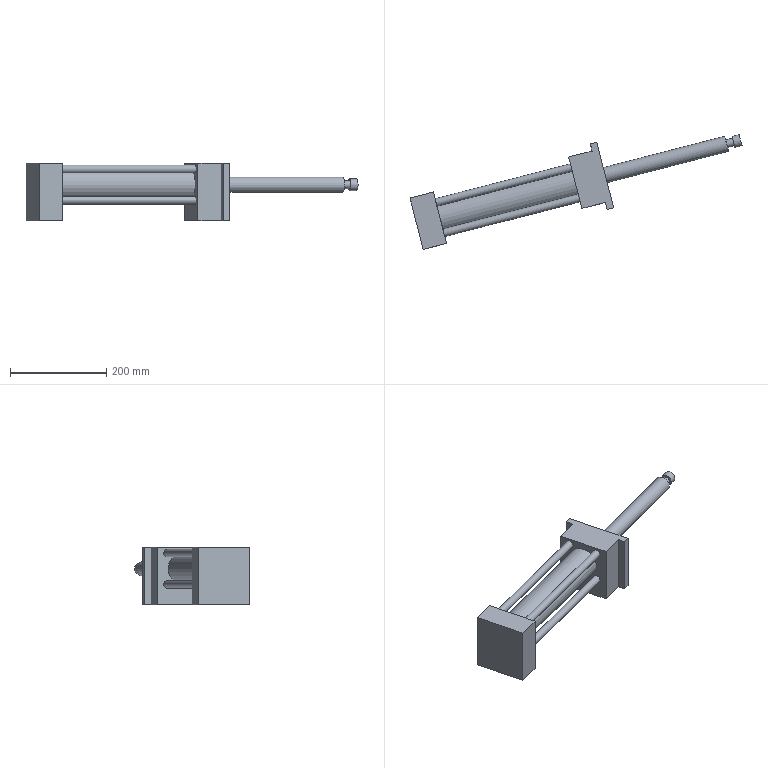Part | STEP file | 车灯-后视镜_id422_x_t | 1 solid | 27 faces | box 688.746 x 238.169 x 120 mm | volume 2911913 mm3 | plane 19 | cylinder 8 | commonest cylinder face diameters 16 x5 24 x1 32 x1 63 x1
STEP:
#1=CARTESIAN_POINT('',(-879.412,-211.845,49.5));
#2=VERTEX_POINT('',#1);
#3=CARTESIAN_POINT('',(-879.412,-211.845,-70.5));
#4=VERTEX_POINT('',#3);
#5=CARTESIAN_POINT('',(-879.412,-211.845,-110.845));
#6=DIRECTION('',(0.,0.,-1.));
#7=VECTOR('',#6,1.);
#8=LINE('',#5,#7);
#9=EDGE_CURVE('',#2,#4,#8,.T.);
#10=ORIENTED_EDGE('',*,*,#9,.T.);
#11=CARTESIAN_POINT('',(-830.995,-199.36,-70.5));
#12=VERTEX_POINT('',#11);
#13=CARTESIAN_POINT('',(-400.091,-88.244,-70.5));
#14=DIRECTION('',(0.9683,0.2497,0.));
#15=VECTOR('',#14,1.);
#16=LINE('',#13,#15);
#17=EDGE_CURVE('',#4,#12,#16,.T.);
#18=ORIENTED_EDGE('',*,*,#17,.T.);
#19=CARTESIAN_POINT('',(-830.995,-199.36,49.5));
#20=VERTEX_POINT('',#19);
#21=CARTESIAN_POINT('',(-830.995,-199.36,-110.845));
#22=DIRECTION('',(0.,0.,-1.));
#23=VECTOR('',#22,1.);
#24=LINE('',#21,#23);
#25=EDGE_CURVE('',#20,#12,#24,.T.);
#26=ORIENTED_EDGE('',*,*,#25,.F.);
#27=CARTESIAN_POINT('',(-400.091,-88.244,49.5));
#28=DIRECTION('',(0.9683,0.2497,0.));
#29=VECTOR('',#28,1.);
#30=LINE('',#27,#29);
#31=EDGE_CURVE('',#2,#20,#30,.T.);
#32=ORIENTED_EDGE('',*,*,#31,.F.);
#33=EDGE_LOOP('',(#10,#18,#26,#32));
#34=FACE_OUTER_BOUND('',#33,.T.);
#35=CARTESIAN_POINT('',(-545.34,-125.699,-110.845));
#36=DIRECTION('',(-0.2497,0.9683,0.));
#37=DIRECTION('',(0.,0.,-1.));
#38=AXIS2_PLACEMENT_3D('',#35,#36,#37);
#39=PLANE('',#38);
#40=ADVANCED_FACE('',(#34),#39,.F.);
#41=CARTESIAN_POINT('',(-906.878,-105.329,49.5));
#42=VERTEX_POINT('',#41);
#43=CARTESIAN_POINT('',(-858.462,-92.844,49.5));
#44=VERTEX_POINT('',#43);
#45=CARTESIAN_POINT('',(-427.558,18.272,49.5));
#46=DIRECTION('',(0.9683,0.2497,0.));
#47=VECTOR('',#46,1.);
#48=LINE('',#45,#47);
#49=EDGE_CURVE('',#42,#44,#48,.T.);
#50=ORIENTED_EDGE('',*,*,#49,.T.);
#51=CARTESIAN_POINT('',(-858.462,-92.844,-70.5));
#52=VERTEX_POINT('',#51);
#53=CARTESIAN_POINT('',(-858.462,-92.844,-110.845));
#54=DIRECTION('',(0.,0.,-1.));
#55=VECTOR('',#54,1.);
#56=LINE('',#53,#55);
#57=EDGE_CURVE('',#44,#52,#56,.T.);
#58=ORIENTED_EDGE('',*,*,#57,.T.);
#59=CARTESIAN_POINT('',(-906.878,-105.329,-70.5));
#60=VERTEX_POINT('',#59);
#61=CARTESIAN_POINT('',(-427.558,18.272,-70.5));
#62=DIRECTION('',(0.9683,0.2497,0.));
#63=VECTOR('',#62,1.);
#64=LINE('',#61,#63);
#65=EDGE_CURVE('',#60,#52,#64,.T.);
#66=ORIENTED_EDGE('',*,*,#65,.F.);
#67=CARTESIAN_POINT('',(-906.878,-105.329,-110.845));
#68=DIRECTION('',(0.,0.,-1.));
#69=VECTOR('',#68,1.);
#70=LINE('',#67,#69);
#71=EDGE_CURVE('',#42,#60,#70,.T.);
#72=ORIENTED_EDGE('',*,*,#71,.F.);
#73=EDGE_LOOP('',(#50,#58,#66,#72));
#74=FACE_OUTER_BOUND('',#73,.T.);
#75=CARTESIAN_POINT('',(-572.807,-19.183,-110.845));
#76=DIRECTION('',(-0.2497,0.9683,0.));
#77=DIRECTION('',(0.,0.,-1.));
#78=AXIS2_PLACEMENT_3D('',#75,#76,#77);
#79=PLANE('',#78);
#80=ADVANCED_FACE('',(#74),#79,.T.);
#81=ORIENTED_EDGE('',*,*,#31,.T.);
#82=CARTESIAN_POINT('',(-844.729,-146.102,49.5));
#83=DIRECTION('',(-0.2497,0.9683,0.));
#84=VECTOR('',#83,1.);
#85=LINE('',#82,#84);
#86=EDGE_CURVE('',#20,#44,#85,.T.);
#87=ORIENTED_EDGE('',*,*,#86,.T.);
#88=ORIENTED_EDGE('',*,*,#49,.F.);
#89=CARTESIAN_POINT('',(-893.145,-158.587,49.5));
#90=DIRECTION('',(-0.2497,0.9683,0.));
#91=VECTOR('',#90,1.);
#92=LINE('',#89,#91);
#93=EDGE_CURVE('',#2,#42,#92,.T.);
#94=ORIENTED_EDGE('',*,*,#93,.F.);
#95=EDGE_LOOP('',(#81,#87,#88,#94));
#96=FACE_OUTER_BOUND('',#95,.T.);
#97=CARTESIAN_POINT('',(-413.825,-34.986,49.5));
#98=DIRECTION('',(0.,0.,1.));
#99=DIRECTION('',(-0.2497,0.9683,0.));
#100=AXIS2_PLACEMENT_3D('',#97,#98,#99);
#101=PLANE('',#100);
#102=ADVANCED_FACE('',(#96),#101,.T.);
#103=CARTESIAN_POINT('',(-893.145,-158.587,-70.5));
#104=DIRECTION('',(-0.2497,0.9683,0.));
#105=VECTOR('',#104,1.);
#106=LINE('',#103,#105);
#107=EDGE_CURVE('',#4,#60,#106,.T.);
#108=ORIENTED_EDGE('',*,*,#107,.T.);
#109=ORIENTED_EDGE('',*,*,#65,.T.);
#110=CARTESIAN_POINT('',(-844.729,-146.102,-70.5));
#111=DIRECTION('',(-0.2497,0.9683,0.));
#112=VECTOR('',#111,1.);
#113=LINE('',#110,#112);
#114=EDGE_CURVE('',#12,#52,#113,.T.);
#115=ORIENTED_EDGE('',*,*,#114,.F.);
#116=ORIENTED_EDGE('',*,*,#17,.F.);
#117=EDGE_LOOP('',(#108,#109,#115,#116));
#118=FACE_OUTER_BOUND('',#117,.T.);
#119=CARTESIAN_POINT('',(-413.825,-34.986,-70.5));
#120=DIRECTION('',(0.,0.,1.));
#121=DIRECTION('',(-0.2497,0.9683,0.));
#122=AXIS2_PLACEMENT_3D('',#119,#120,#121);
#123=PLANE('',#122);
#124=ADVANCED_FACE('',(#118),#123,.F.);
#125=CARTESIAN_POINT('',(-533.02,6.744,49.5));
#126=VERTEX_POINT('',#125);
#127=CARTESIAN_POINT('',(-533.02,6.744,-70.5));
#128=VERTEX_POINT('',#127);
#129=CARTESIAN_POINT('',(-533.02,6.744,-36.5));
#130=DIRECTION('',(0.,0.,-1.));
#131=VECTOR('',#130,1.);
#132=LINE('',#129,#131);
#133=EDGE_CURVE('',#126,#128,#132,.T.);
#134=ORIENTED_EDGE('',*,*,#133,.T.);
#135=CARTESIAN_POINT('',(-529.232,-7.946,-70.5));
#136=VERTEX_POINT('',#135);
#137=CARTESIAN_POINT('',(-515.499,-61.204,-70.5));
#138=DIRECTION('',(0.2497,-0.9683,0.));
#139=VECTOR('',#138,1.);
#140=LINE('',#137,#139);
#141=EDGE_CURVE('',#128,#136,#140,.T.);
#142=ORIENTED_EDGE('',*,*,#141,.T.);
#143=CARTESIAN_POINT('',(-529.232,-7.946,49.5));
#144=VERTEX_POINT('',#143);
#145=CARTESIAN_POINT('',(-529.232,-7.946,-36.5));
#146=DIRECTION('',(0.,0.,-1.));
#147=VECTOR('',#146,1.);
#148=LINE('',#145,#147);
#149=EDGE_CURVE('',#144,#136,#148,.T.);
#150=ORIENTED_EDGE('',*,*,#149,.F.);
#151=CARTESIAN_POINT('',(-515.499,-61.204,49.5));
#152=DIRECTION('',(0.2497,-0.9683,0.));
#153=VECTOR('',#152,1.);
#154=LINE('',#151,#153);
#155=EDGE_CURVE('',#126,#144,#154,.T.);
#156=ORIENTED_EDGE('',*,*,#155,.F.);
#157=EDGE_LOOP('',(#134,#142,#150,#156));
#158=FACE_OUTER_BOUND('',#157,.T.);
#159=CARTESIAN_POINT('',(-526.735,-17.63,-36.5));
#160=DIRECTION('',(0.9683,0.2497,0.));
#161=DIRECTION('',(0.,0.,-1.));
#162=AXIS2_PLACEMENT_3D('',#159,#160,#161);
#163=PLANE('',#162);
#164=ADVANCED_FACE('',(#158),#163,.F.);
#165=CARTESIAN_POINT('',(-850.846,-122.378,37.));
#166=VERTEX_POINT('',#165);
#167=CARTESIAN_POINT('',(-852.844,-114.631,37.));
#168=DIRECTION('',(-0.9683,-0.2497,0.));
#169=DIRECTION('',(0.2497,-0.9683,0.));
#170=AXIS2_PLACEMENT_3D('',#167,#168,#169);
#171=CIRCLE('',#170,8.);
#172=EDGE_CURVE('',#166,#166,#171,.T.);
#173=ORIENTED_EDGE('',*,*,#172,.T.);
#174=EDGE_LOOP('',(#173));
#175=FACE_BOUND('',#174,.T.);
#176=CARTESIAN_POINT('',(-836.863,-176.604,4.5));
#177=VERTEX_POINT('',#176);
#178=CARTESIAN_POINT('',(-844.729,-146.102,4.5));
#179=DIRECTION('',(-0.9683,-0.2497,0.));
#180=DIRECTION('',(0.2497,-0.9683,0.));
#181=AXIS2_PLACEMENT_3D('',#178,#179,#180);
#182=CIRCLE('',#181,31.5);
#183=EDGE_CURVE('',#177,#177,#182,.T.);
#184=ORIENTED_EDGE('',*,*,#183,.T.);
#185=EDGE_LOOP('',(#184));
#186=FACE_BOUND('',#185,.T.);
#187=CARTESIAN_POINT('',(-850.846,-122.378,-28.));
#188=VERTEX_POINT('',#187);
#189=CARTESIAN_POINT('',(-852.844,-114.631,-28.));
#190=DIRECTION('',(-0.9683,-0.2497,0.));
#191=DIRECTION('',(0.2497,-0.9683,0.));
#192=AXIS2_PLACEMENT_3D('',#189,#190,#191);
#193=CIRCLE('',#192,8.);
#194=EDGE_CURVE('',#188,#188,#193,.T.);
#195=ORIENTED_EDGE('',*,*,#194,.T.);
#196=EDGE_LOOP('',(#195));
#197=FACE_BOUND('',#196,.T.);
#198=CARTESIAN_POINT('',(-834.616,-185.319,-28.));
#199=VERTEX_POINT('',#198);
#200=CARTESIAN_POINT('',(-836.614,-177.572,-28.));
#201=DIRECTION('',(-0.9683,-0.2497,0.));
#202=DIRECTION('',(0.2497,-0.9683,0.));
#203=AXIS2_PLACEMENT_3D('',#200,#201,#202);
#204=CIRCLE('',#203,8.);
#205=EDGE_CURVE('',#199,#199,#204,.T.);
#206=ORIENTED_EDGE('',*,*,#205,.T.);
#207=EDGE_LOOP('',(#206));
#208=FACE_BOUND('',#207,.T.);
#209=CARTESIAN_POINT('',(-834.616,-185.319,37.));
#210=VERTEX_POINT('',#209);
#211=CARTESIAN_POINT('',(-836.614,-177.572,37.));
#212=DIRECTION('',(-0.9683,-0.2497,0.));
#213=DIRECTION('',(0.2497,-0.9683,0.));
#214=AXIS2_PLACEMENT_3D('',#211,#212,#213);
#215=CIRCLE('',#214,8.);
#216=EDGE_CURVE('',#210,#210,#215,.T.);
#217=ORIENTED_EDGE('',*,*,#216,.T.);
#218=EDGE_LOOP('',(#217));
#219=FACE_BOUND('',#218,.T.);
#220=ORIENTED_EDGE('',*,*,#25,.T.);
#221=ORIENTED_EDGE('',*,*,#114,.T.);
#222=ORIENTED_EDGE('',*,*,#57,.F.);
#223=ORIENTED_EDGE('',*,*,#86,.F.);
#224=EDGE_LOOP('',(#220,#221,#222,#223));
#225=FACE_BOUND('',#224,.T.);
#226=CARTESIAN_POINT('',(-844.729,-146.102,-110.845));
#227=DIRECTION('',(-0.9683,-0.2497,0.));
#228=DIRECTION('',(0.,0.,1.));
#229=AXIS2_PLACEMENT_3D('',#226,#227,#228);
#230=PLANE('',#229);
#231=ADVANCED_FACE('',(#175,#186,#197,#208,#219,#225),#230,.F.);
#232=CARTESIAN_POINT('',(-557.797,-97.413,37.));
#233=VERTEX_POINT('',#232);
#234=CARTESIAN_POINT('',(-555.8,-105.16,37.));
#235=DIRECTION('',(0.9683,0.2497,0.));
#236=DIRECTION('',(-0.2497,0.9683,0.));
#237=AXIS2_PLACEMENT_3D('',#234,#235,#236);
#238=CIRCLE('',#237,8.);
#239=EDGE_CURVE('',#233,#233,#238,.T.);
#240=ORIENTED_EDGE('',*,*,#239,.F.);
#241=EDGE_LOOP('',(#240));
#242=FACE_BOUND('',#241,.T.);
#243=ORIENTED_EDGE('',*,*,#216,.F.);
#244=EDGE_LOOP('',(#243));
#245=FACE_BOUND('',#244,.T.);
#246=CARTESIAN_POINT('',(-807.564,-170.081,37.));
#247=DIRECTION('',(0.9683,0.2497,0.));
#248=DIRECTION('',(-0.2497,0.9683,0.));
#249=AXIS2_PLACEMENT_3D('',#246,#247,#248);
#250=CYLINDRICAL_SURFACE('',#249,8.);
#251=ADVANCED_FACE('',(#242,#245),#250,.T.);
#252=CARTESIAN_POINT('',(-557.797,-97.413,-28.));
#253=VERTEX_POINT('',#252);
#254=CARTESIAN_POINT('',(-555.8,-105.16,-28.));
#255=DIRECTION('',(0.9683,0.2497,0.));
#256=DIRECTION('',(-0.2497,0.9683,0.));
#257=AXIS2_PLACEMENT_3D('',#254,#255,#256);
#258=CIRCLE('',#257,8.);
#259=EDGE_CURVE('',#253,#253,#258,.T.);
#260=ORIENTED_EDGE('',*,*,#259,.F.);
#261=EDGE_LOOP('',(#260));
#262=FACE_BOUND('',#261,.T.);
#263=ORIENTED_EDGE('',*,*,#205,.F.);
#264=EDGE_LOOP('',(#263));
#265=FACE_BOUND('',#264,.T.);
#266=CARTESIAN_POINT('',(-807.564,-170.081,-28.));
#267=DIRECTION('',(0.9683,0.2497,0.));
#268=DIRECTION('',(-0.2497,0.9683,0.));
#269=AXIS2_PLACEMENT_3D('',#266,#267,#268);
#270=CYLINDRICAL_SURFACE('',#269,8.);
#271=ADVANCED_FACE('',(#262,#265),#270,.T.);
#272=CARTESIAN_POINT('',(-574.028,-34.472,-28.));
#273=VERTEX_POINT('',#272);
#274=CARTESIAN_POINT('',(-572.03,-42.219,-28.));
#275=DIRECTION('',(0.9683,0.2497,0.));
#276=DIRECTION('',(-0.2497,0.9683,0.));
#277=AXIS2_PLACEMENT_3D('',#274,#275,#276);
#278=CIRCLE('',#277,8.);
#279=EDGE_CURVE('',#273,#273,#278,.T.);
#280=ORIENTED_EDGE('',*,*,#279,.F.);
#281=EDGE_LOOP('',(#280));
#282=FACE_BOUND('',#281,.T.);
#283=ORIENTED_EDGE('',*,*,#194,.F.);
#284=EDGE_LOOP('',(#283));
#285=FACE_BOUND('',#284,.T.);
#286=CARTESIAN_POINT('',(-823.794,-107.14,-28.));
#287=DIRECTION('',(0.9683,0.2497,0.));
#288=DIRECTION('',(-0.2497,0.9683,0.));
#289=AXIS2_PLACEMENT_3D('',#286,#287,#288);
#290=CYLINDRICAL_SURFACE('',#289,8.);
#291=ADVANCED_FACE('',(#282,#285),#290,.T.);
#292=CARTESIAN_POINT('',(-571.781,-43.187,4.5));
#293=VERTEX_POINT('',#292);
#294=CARTESIAN_POINT('',(-563.915,-73.689,4.5));
#295=DIRECTION('',(0.9683,0.2497,0.));
#296=DIRECTION('',(-0.2497,0.9683,0.));
#297=AXIS2_PLACEMENT_3D('',#294,#295,#296);
#298=CIRCLE('',#297,31.5);
#299=EDGE_CURVE('',#293,#293,#298,.T.);
#300=ORIENTED_EDGE('',*,*,#299,.F.);
#301=EDGE_LOOP('',(#300));
#302=FACE_BOUND('',#301,.T.);
#303=ORIENTED_EDGE('',*,*,#183,.F.);
#304=EDGE_LOOP('',(#303));
#305=FACE_BOUND('',#304,.T.);
#306=CARTESIAN_POINT('',(-559.073,-72.441,4.5));
#307=DIRECTION('',(-0.9683,-0.2497,0.));
#308=DIRECTION('',(0.2497,-0.9683,0.));
#309=AXIS2_PLACEMENT_3D('',#306,#307,#308);
#310=CYLINDRICAL_SURFACE('',#309,31.5);
#311=ADVANCED_FACE('',(#302,#305),#310,.T.);
#312=CARTESIAN_POINT('',(-574.028,-34.472,37.));
#313=VERTEX_POINT('',#312);
#314=CARTESIAN_POINT('',(-572.03,-42.219,37.));
#315=DIRECTION('',(0.9683,0.2497,0.));
#316=DIRECTION('',(-0.2497,0.9683,0.));
#317=AXIS2_PLACEMENT_3D('',#314,#315,#316);
#318=CIRCLE('',#317,8.);
#319=EDGE_CURVE('',#313,#313,#318,.T.);
#320=ORIENTED_EDGE('',*,*,#319,.F.);
#321=EDGE_LOOP('',(#320));
#322=FACE_BOUND('',#321,.T.);
#323=ORIENTED_EDGE('',*,*,#172,.F.);
#324=EDGE_LOOP('',(#323));
#325=FACE_BOUND('',#324,.T.);
#326=CARTESIAN_POINT('',(-823.794,-107.14,37.));
#327=DIRECTION('',(0.9683,0.2497,0.));
#328=DIRECTION('',(-0.2497,0.9683,0.));
#329=AXIS2_PLACEMENT_3D('',#326,#327,#328);
#330=CYLINDRICAL_SURFACE('',#329,8.);
#331=ADVANCED_FACE('',(#322,#325),#330,.T.);
#332=CARTESIAN_POINT('',(-550.182,-126.947,49.5));
#333=VERTEX_POINT('',#332);
#334=CARTESIAN_POINT('',(-550.182,-126.947,-70.5));
#335=VERTEX_POINT('',#334);
#336=CARTESIAN_POINT('',(-550.182,-126.947,-110.845));
#337=DIRECTION('',(0.,0.,-1.));
#338=VECTOR('',#337,1.);
#339=LINE('',#336,#338);
#340=EDGE_CURVE('',#333,#335,#339,.T.);
#341=ORIENTED_EDGE('',*,*,#340,.T.);
#342=CARTESIAN_POINT('',(-501.765,-114.462,-70.5));
#343=VERTEX_POINT('',#342);
#344=CARTESIAN_POINT('',(-158.011,-25.819,-70.5));
#345=DIRECTION('',(0.9683,0.2497,0.));
#346=VECTOR('',#345,1.);
#347=LINE('',#344,#346);
#348=EDGE_CURVE('',#335,#343,#347,.T.);
#349=ORIENTED_EDGE('',*,*,#348,.T.);
#350=CARTESIAN_POINT('',(-501.765,-114.462,49.5));
#351=VERTEX_POINT('',#350);
#352=CARTESIAN_POINT('',(-501.765,-114.462,-36.5));
#353=DIRECTION('',(0.,0.,-1.));
#354=VECTOR('',#353,1.);
#355=LINE('',#352,#354);
#356=EDGE_CURVE('',#351,#343,#355,.T.);
#357=ORIENTED_EDGE('',*,*,#356,.F.);
#358=CARTESIAN_POINT('',(-158.011,-25.819,49.5));
#359=DIRECTION('',(0.9683,0.2497,0.));
#360=VECTOR('',#359,1.);
#361=LINE('',#358,#360);
#362=EDGE_CURVE('',#333,#351,#361,.T.);
#363=ORIENTED_EDGE('',*,*,#362,.F.);
#364=EDGE_LOOP('',(#341,#349,#357,#363));
#365=FACE_OUTER_BOUND('',#364,.T.);
#366=CARTESIAN_POINT('',(-303.259,-63.274,-110.845));
#367=DIRECTION('',(-0.2497,0.9683,0.));
#368=DIRECTION('',(0.,0.,-1.));
#369=AXIS2_PLACEMENT_3D('',#366,#367,#368);
#370=PLANE('',#369);
#371=ADVANCED_FACE('',(#365),#370,.F.);
#372=ORIENTED_EDGE('',*,*,#239,.T.);
#373=EDGE_LOOP('',(#372));
#374=FACE_BOUND('',#373,.T.);
#375=ORIENTED_EDGE('',*,*,#259,.T.);
#376=EDGE_LOOP('',(#375));
#377=FACE_BOUND('',#376,.T.);
#378=ORIENTED_EDGE('',*,*,#279,.T.);
#379=EDGE_LOOP('',(#378));
#380=FACE_BOUND('',#379,.T.);
#381=ORIENTED_EDGE('',*,*,#299,.T.);
#382=EDGE_LOOP('',(#381));
#383=FACE_BOUND('',#382,.T.);
#384=ORIENTED_EDGE('',*,*,#319,.T.);
#385=EDGE_LOOP('',(#384));
#386=FACE_BOUND('',#385,.T.);
#387=CARTESIAN_POINT('',(-577.648,-20.431,-70.5));
#388=VERTEX_POINT('',#387);
#389=CARTESIAN_POINT('',(-563.915,-73.689,-70.5));
#390=DIRECTION('',(-0.2497,0.9683,0.));
#391=VECTOR('',#390,1.);
#392=LINE('',#389,#391);
#393=EDGE_CURVE('',#335,#388,#392,.T.);
#394=ORIENTED_EDGE('',*,*,#393,.F.);
#395=ORIENTED_EDGE('',*,*,#340,.F.);
#396=CARTESIAN_POINT('',(-577.648,-20.431,49.5));
#397=VERTEX_POINT('',#396);
#398=CARTESIAN_POINT('',(-563.915,-73.689,49.5));
#399=DIRECTION('',(-0.2497,0.9683,0.));
#400=VECTOR('',#399,1.);
#401=LINE('',#398,#400);
#402=EDGE_CURVE('',#333,#397,#401,.T.);
#403=ORIENTED_EDGE('',*,*,#402,.T.);
#404=CARTESIAN_POINT('',(-577.648,-20.431,-110.845));
#405=DIRECTION('',(0.,0.,-1.));
#406=VECTOR('',#405,1.);
#407=LINE('',#404,#406);
#408=EDGE_CURVE('',#397,#388,#407,.T.);
#409=ORIENTED_EDGE('',*,*,#408,.T.);
#410=EDGE_LOOP('',(#394,#395,#403,#409));
#411=FACE_BOUND('',#410,.T.);
#412=CARTESIAN_POINT('',(-563.915,-73.689,-110.845));
#413=DIRECTION('',(-0.9683,-0.2497,0.));
#414=DIRECTION('',(0.,0.,1.));
#415=AXIS2_PLACEMENT_3D('',#412,#413,#414);
#416=PLANE('',#415);
#417=ADVANCED_FACE('',(#374,#377,#380,#383,#386,#411),#416,.T.);
#418=CARTESIAN_POINT('',(-185.477,80.697,-70.5));
#419=DIRECTION('',(0.9683,0.2497,0.));
#420=VECTOR('',#419,1.);
#421=LINE('',#418,#420);
#422=EDGE_CURVE('',#388,#136,#421,.T.);
#423=ORIENTED_EDGE('',*,*,#422,.F.);
#424=ORIENTED_EDGE('',*,*,#408,.F.);
#425=CARTESIAN_POINT('',(-185.477,80.697,49.5));
#426=DIRECTION('',(0.9683,0.2497,0.));
#427=VECTOR('',#426,1.);
#428=LINE('',#425,#427);
#429=EDGE_CURVE('',#397,#144,#428,.T.);
#430=ORIENTED_EDGE('',*,*,#429,.T.);
#431=ORIENTED_EDGE('',*,*,#149,.T.);
#432=EDGE_LOOP('',(#423,#424,#430,#431));
#433=FACE_OUTER_BOUND('',#432,.T.);
#434=CARTESIAN_POINT('',(-330.726,43.242,-110.845));
#435=DIRECTION('',(-0.2497,0.9683,0.));
#436=DIRECTION('',(0.,0.,-1.));
#437=AXIS2_PLACEMENT_3D('',#434,#435,#436);
#438=PLANE('',#437);
#439=ADVANCED_FACE('',(#433),#438,.T.);
#440=ORIENTED_EDGE('',*,*,#402,.F.);
#441=ORIENTED_EDGE('',*,*,#362,.T.);
#442=CARTESIAN_POINT('',(-497.977,-129.152,49.5));
#443=VERTEX_POINT('',#442);
#444=CARTESIAN_POINT('',(-515.499,-61.204,49.5));
#445=DIRECTION('',(0.2497,-0.9683,0.));
#446=VECTOR('',#445,1.);
#447=LINE('',#444,#446);
#448=EDGE_CURVE('',#351,#443,#447,.T.);
#449=ORIENTED_EDGE('',*,*,#448,.T.);
#450=CARTESIAN_POINT('',(-484.421,-125.657,49.5));
#451=VERTEX_POINT('',#450);
#452=CARTESIAN_POINT('',(-154.222,-40.509,49.5));
#453=DIRECTION('',(0.9683,0.2497,0.));
#454=VECTOR('',#453,1.);
#455=LINE('',#452,#454);
#456=EDGE_CURVE('',#443,#451,#455,.T.);
#457=ORIENTED_EDGE('',*,*,#456,.T.);
#458=CARTESIAN_POINT('',(-519.464,10.24,49.5));
#459=VERTEX_POINT('',#458);
#460=CARTESIAN_POINT('',(-501.942,-57.708,49.5));
#461=DIRECTION('',(0.2497,-0.9683,0.));
#462=VECTOR('',#461,1.);
#463=LINE('',#460,#462);
#464=EDGE_CURVE('',#459,#451,#463,.T.);
#465=ORIENTED_EDGE('',*,*,#464,.F.);
#466=CARTESIAN_POINT('',(-557.229,0.5014,49.5));
#467=DIRECTION('',(0.9683,0.2497,0.));
#468=VECTOR('',#467,1.);
#469=LINE('',#466,#468);
#470=EDGE_CURVE('',#126,#459,#469,.T.);
#471=ORIENTED_EDGE('',*,*,#470,.F.);
#472=ORIENTED_EDGE('',*,*,#155,.T.);
#473=ORIENTED_EDGE('',*,*,#429,.F.);
#474=EDGE_LOOP('',(#440,#441,#449,#457,#465,#471,#472,#473));
#475=FACE_OUTER_BOUND('',#474,.T.);
#476=CARTESIAN_POINT('',(-171.744,27.439,49.5));
#477=DIRECTION('',(0.,0.,1.));
#478=DIRECTION('',(-0.2497,0.9683,0.));
#479=AXIS2_PLACEMENT_3D('',#476,#477,#478);
#480=PLANE('',#479);
#481=ADVANCED_FACE('',(#475),#480,.T.);
#482=ORIENTED_EDGE('',*,*,#348,.F.);
#483=ORIENTED_EDGE('',*,*,#393,.T.);
#484=ORIENTED_EDGE('',*,*,#422,.T.);
#485=ORIENTED_EDGE('',*,*,#141,.F.);
#486=CARTESIAN_POINT('',(-519.464,10.24,-70.5));
#487=VERTEX_POINT('',#486);
#488=CARTESIAN_POINT('',(-189.266,95.387,-70.5));
#489=DIRECTION('',(0.9683,0.2497,0.));
#490=VECTOR('',#489,1.);
#491=LINE('',#488,#490);
#492=EDGE_CURVE('',#128,#487,#491,.T.);
#493=ORIENTED_EDGE('',*,*,#492,.T.);
#494=CARTESIAN_POINT('',(-484.421,-125.657,-70.5));
#495=VERTEX_POINT('',#494);
#496=CARTESIAN_POINT('',(-501.942,-57.708,-70.5));
#497=DIRECTION('',(0.2497,-0.9683,0.));
#498=VECTOR('',#497,1.);
#499=LINE('',#496,#498);
#500=EDGE_CURVE('',#487,#495,#499,.T.);
#501=ORIENTED_EDGE('',*,*,#500,.T.);
#502=CARTESIAN_POINT('',(-497.977,-129.152,-70.5));
#503=VERTEX_POINT('',#502);
#504=CARTESIAN_POINT('',(-154.222,-40.509,-70.5));
#505=DIRECTION('',(0.9683,0.2497,0.));
#506=VECTOR('',#505,1.);
#507=LINE('',#504,#506);
#508=EDGE_CURVE('',#503,#495,#507,.T.);
#509=ORIENTED_EDGE('',*,*,#508,.F.);
#510=CARTESIAN_POINT('',(-515.499,-61.204,-70.5));
#511=DIRECTION('',(0.2497,-0.9683,0.));
#512=VECTOR('',#511,1.);
#513=LINE('',#510,#512);
#514=EDGE_CURVE('',#343,#503,#513,.T.);
#515=ORIENTED_EDGE('',*,*,#514,.F.);
#516=EDGE_LOOP('',(#482,#483,#484,#485,#493,#501,#509,#515));
#517=FACE_OUTER_BOUND('',#516,.T.);
#518=CARTESIAN_POINT('',(-171.744,27.439,-70.5));
#519=DIRECTION('',(0.,0.,1.));
#520=DIRECTION('',(-0.2497,0.9683,0.));
#521=AXIS2_PLACEMENT_3D('',#518,#519,#520);
#522=PLANE('',#521);
#523=ADVANCED_FACE('',(#517),#522,.F.);
#524=ORIENTED_EDGE('',*,*,#492,.F.);
#525=ORIENTED_EDGE('',*,*,#133,.F.);
#526=ORIENTED_EDGE('',*,*,#470,.T.);
#527=CARTESIAN_POINT('',(-519.464,10.24,-36.5));
#528=DIRECTION('',(0.,0.,-1.));
#529=VECTOR('',#528,1.);
#530=LINE('',#527,#529);
#531=EDGE_CURVE('',#459,#487,#530,.T.);
#532=ORIENTED_EDGE('',*,*,#531,.T.);
#533=EDGE_LOOP('',(#524,#525,#526,#532));
#534=FACE_OUTER_BOUND('',#533,.T.);
#535=CARTESIAN_POINT('',(-557.229,0.5014,53.5));
#536=DIRECTION('',(-0.2497,0.9683,0.));
#537=DIRECTION('',(0.,0.,-1.));
#538=AXIS2_PLACEMENT_3D('',#535,#536,#537);
#539=PLANE('',#538);
#540=ADVANCED_FACE('',(#534),#539,.T.);
#541=CARTESIAN_POINT('',(-497.977,-129.152,-36.5));
#542=DIRECTION('',(0.,0.,-1.));
#543=VECTOR('',#542,1.);
#544=LINE('',#541,#543);
#545=EDGE_CURVE('',#443,#503,#544,.T.);
#546=ORIENTED_EDGE('',*,*,#545,.T.);
#547=ORIENTED_EDGE('',*,*,#508,.T.);
#548=CARTESIAN_POINT('',(-484.421,-125.657,-36.5));
#549=DIRECTION('',(0.,0.,-1.));
#550=VECTOR('',#549,1.);
#551=LINE('',#548,#550);
#552=EDGE_CURVE('',#451,#495,#551,.T.);
#553=ORIENTED_EDGE('',*,*,#552,.F.);
#554=ORIENTED_EDGE('',*,*,#456,.F.);
#555=EDGE_LOOP('',(#546,#547,#553,#554));
#556=FACE_OUTER_BOUND('',#555,.T.);
#557=CARTESIAN_POINT('',(-522.185,-135.395,53.5));
#558=DIRECTION('',(-0.2497,0.9683,0.));
#559=DIRECTION('',(0.,0.,-1.));
#560=AXIS2_PLACEMENT_3D('',#557,#558,#559);
#561=PLANE('',#560);
#562=ADVANCED_FACE('',(#556),#561,.F.);
#563=ORIENTED_EDGE('',*,*,#500,.F.);
#564=ORIENTED_EDGE('',*,*,#531,.F.);
#565=ORIENTED_EDGE('',*,*,#464,.T.);
#566=ORIENTED_EDGE('',*,*,#552,.T.);
#567=EDGE_LOOP('',(#563,#564,#565,#566));
#568=FACE_BOUND('',#567,.T.);
#569=CARTESIAN_POINT('',(-505.937,-42.215,4.5));
#570=VERTEX_POINT('',#569);
#571=CARTESIAN_POINT('',(-501.942,-57.708,4.5));
#572=DIRECTION('',(0.9683,0.2497,0.));
#573=DIRECTION('',(-0.2497,0.9683,0.));
#574=AXIS2_PLACEMENT_3D('',#571,#572,#573);
#575=CIRCLE('',#574,16.);
#576=EDGE_CURVE('',#570,#570,#575,.T.);
#577=ORIENTED_EDGE('',*,*,#576,.F.);
#578=EDGE_LOOP('',(#577));
#579=FACE_BOUND('',#578,.T.);
#580=CARTESIAN_POINT('',(-513.179,-14.134,-36.5));
#581=DIRECTION('',(0.9683,0.2497,0.));
#582=DIRECTION('',(0.,0.,-1.));
#583=AXIS2_PLACEMENT_3D('',#580,#581,#582);
#584=PLANE('',#583);
#585=ADVANCED_FACE('',(#568,#579),#584,.T.);
#586=ORIENTED_EDGE('',*,*,#356,.T.);
#587=ORIENTED_EDGE('',*,*,#514,.T.);
#588=ORIENTED_EDGE('',*,*,#545,.F.);
#589=ORIENTED_EDGE('',*,*,#448,.F.);
#590=EDGE_LOOP('',(#586,#587,#588,#589));
#591=FACE_OUTER_BOUND('',#590,.T.);
#592=CARTESIAN_POINT('',(-526.735,-17.63,-36.5));
#593=DIRECTION('',(0.9683,0.2497,0.));
#594=DIRECTION('',(0.,0.,-1.));
#595=AXIS2_PLACEMENT_3D('',#592,#593,#594);
#596=PLANE('',#595);
#597=ADVANCED_FACE('',(#591),#596,.F.);
#598=CARTESIAN_POINT('',(-254.173,22.706,4.5));
#599=VERTEX_POINT('',#598);
#600=CARTESIAN_POINT('',(-250.178,7.213,4.5));
#601=DIRECTION('',(0.9683,0.2497,0.));
#602=DIRECTION('',(-0.2497,0.9683,0.));
#603=AXIS2_PLACEMENT_3D('',#600,#601,#602);
#604=CIRCLE('',#603,16.);
#605=EDGE_CURVE('',#599,#599,#604,.T.);
#606=ORIENTED_EDGE('',*,*,#605,.F.);
#607=EDGE_LOOP('',(#606));
#608=FACE_BOUND('',#607,.T.);
#609=ORIENTED_EDGE('',*,*,#576,.T.);
#610=EDGE_LOOP('',(#609));
#611=FACE_BOUND('',#610,.T.);
#612=CARTESIAN_POINT('',(-476.766,-51.216,4.5));
#613=DIRECTION('',(-0.9683,-0.2497,0.));
#614=DIRECTION('',(0.,0.,-1.));
#615=AXIS2_PLACEMENT_3D('',#612,#613,#614);
#616=CYLINDRICAL_SURFACE('',#615,16.);
#617=ADVANCED_FACE('',(#608,#611),#616,.T.);
#618=CARTESIAN_POINT('',(-252.176,14.96,4.5));
#619=VERTEX_POINT('',#618);
#620=CARTESIAN_POINT('',(-250.178,7.213,4.5));
#621=DIRECTION('',(0.9683,0.2497,0.));
#622=DIRECTION('',(-0.2497,0.9683,0.));
#623=AXIS2_PLACEMENT_3D('',#620,#621,#622);
#624=CIRCLE('',#623,8.);
#625=EDGE_CURVE('',#619,#619,#624,.T.);
#626=ORIENTED_EDGE('',*,*,#625,.F.);
#627=EDGE_LOOP('',(#626));
#628=FACE_BOUND('',#627,.T.);
#629=ORIENTED_EDGE('',*,*,#605,.T.);
#630=EDGE_LOOP('',(#629));
#631=FACE_BOUND('',#630,.T.);
#632=CARTESIAN_POINT('',(-250.178,7.213,4.5));
#633=DIRECTION('',(0.9683,0.2497,0.));
#634=DIRECTION('',(0.,0.,1.));
#635=AXIS2_PLACEMENT_3D('',#632,#633,#634);
#636=PLANE('',#635);
#637=ADVANCED_FACE('',(#628,#631),#636,.T.);
#638=ORIENTED_EDGE('',*,*,#625,.T.);
#639=EDGE_LOOP('',(#638));
#640=FACE_BOUND('',#639,.T.);
#641=CARTESIAN_POINT('',(-235.653,10.959,-3.5));
#642=VERTEX_POINT('',#641);
#643=CARTESIAN_POINT('',(-235.653,10.959,4.5));
#644=DIRECTION('',(0.9683,0.2497,0.));
#645=DIRECTION('',(0.,0.,-1.));
#646=AXIS2_PLACEMENT_3D('',#643,#644,#645);
#647=CIRCLE('',#646,8.);
#648=EDGE_CURVE('',#642,#642,#647,.T.);
#649=ORIENTED_EDGE('',*,*,#648,.F.);
#650=EDGE_LOOP('',(#649));
#651=FACE_BOUND('',#650,.T.);
#652=CARTESIAN_POINT('',(-281.165,-0.7772,4.5));
#653=DIRECTION('',(0.9683,0.2497,0.));
#654=DIRECTION('',(0.,0.,1.));
#655=AXIS2_PLACEMENT_3D('',#652,#653,#654);
#656=CYLINDRICAL_SURFACE('',#655,8.);
#657=ADVANCED_FACE('',(#640,#651),#656,.T.);
#658=CARTESIAN_POINT('',(-221.128,14.704,16.5));
#659=VERTEX_POINT('',#658);
#660=CARTESIAN_POINT('',(-221.128,14.704,4.5));
#661=DIRECTION('',(-0.9683,-0.2497,0.));
#662=DIRECTION('',(0.,0.,1.));
#663=AXIS2_PLACEMENT_3D('',#660,#661,#662);
#664=CIRCLE('',#663,12.);
#665=EDGE_CURVE('',#659,#659,#664,.T.);
#666=ORIENTED_EDGE('',*,*,#665,.F.);
#667=EDGE_LOOP('',(#666));
#668=FACE_OUTER_BOUND('',#667,.T.);
#669=CARTESIAN_POINT('',(-221.128,14.704,4.5));
#670=DIRECTION('',(0.9683,0.2497,0.));
#671=DIRECTION('',(0.,0.,1.));
#672=AXIS2_PLACEMENT_3D('',#669,#670,#671);
#673=PLANE('',#672);
#674=ADVANCED_FACE('',(#668),#673,.T.);
#675=ORIENTED_EDGE('',*,*,#648,.T.);
#676=EDGE_LOOP('',(#675));
#677=FACE_BOUND('',#676,.T.);
#678=CARTESIAN_POINT('',(-235.653,10.959,-7.5));
#679=VERTEX_POINT('',#678);
#680=CARTESIAN_POINT('',(-235.653,10.959,4.5));
#681=DIRECTION('',(0.9683,0.2497,0.));
#682=DIRECTION('',(0.,0.,-1.));
#683=AXIS2_PLACEMENT_3D('',#680,#681,#682);
#684=CIRCLE('',#683,12.);
#685=EDGE_CURVE('',#679,#679,#684,.T.);
#686=ORIENTED_EDGE('',*,*,#685,.F.);
#687=EDGE_LOOP('',(#686));
#688=FACE_BOUND('',#687,.T.);
#689=CARTESIAN_POINT('',(-235.653,10.959,4.5));
#690=DIRECTION('',(-0.9683,-0.2497,0.));
#691=DIRECTION('',(0.,0.,-1.));
#692=AXIS2_PLACEMENT_3D('',#689,#690,#691);
#693=PLANE('',#692);
#694=ADVANCED_FACE('',(#677,#688),#693,.T.);
#695=ORIENTED_EDGE('',*,*,#665,.T.);
#696=EDGE_LOOP('',(#695));
#697=FACE_BOUND('',#696,.T.);
#698=ORIENTED_EDGE('',*,*,#685,.T.);
#699=EDGE_LOOP('',(#698));
#700=FACE_BOUND('',#699,.T.);
#701=CARTESIAN_POINT('',(-232.748,11.708,4.5));
#702=DIRECTION('',(0.9683,0.2497,0.));
#703=DIRECTION('',(0.,0.,1.));
#704=AXIS2_PLACEMENT_3D('',#701,#702,#703);
#705=CYLINDRICAL_SURFACE('',#704,12.);
#706=ADVANCED_FACE('',(#697,#700),#705,.T.);
#707=ORIENTED_EDGE('',*,*,#93,.T.);
#708=ORIENTED_EDGE('',*,*,#71,.T.);
#709=ORIENTED_EDGE('',*,*,#107,.F.);
#710=ORIENTED_EDGE('',*,*,#9,.F.);
#711=EDGE_LOOP('',(#707,#708,#709,#710));
#712=FACE_OUTER_BOUND('',#711,.T.);
#713=CARTESIAN_POINT('',(-951.972,69.544,14.5));
#714=DIRECTION('',(-0.9683,-0.2497,0.));
#715=DIRECTION('',(0.,0.,1.));
#716=AXIS2_PLACEMENT_3D('',#713,#714,#715);
#717=PLANE('',#716);
#718=ADVANCED_FACE('',(#712),#717,.T.);
#719=CLOSED_SHELL('',(#40,#80,#102,#124,#164,#231,#251,#271,#291,#311,#331,#371,#417,#439,#481,#523,#540,#562,#585,#597,#617,#637,#657,#674,#694,#706,#718));
#720=MANIFOLD_SOLID_BREP('',#719);
#721=(LENGTH_UNIT()NAMED_UNIT(*)SI_UNIT(.MILLI.,.METRE.));
#722=UNCERTAINTY_MEASURE_WITH_UNIT(LENGTH_MEASURE(0.00002),#721,'','');
#723=(NAMED_UNIT(*)PLANE_ANGLE_UNIT()SI_UNIT($,.RADIAN.));
#724=PLANE_ANGLE_MEASURE_WITH_UNIT(PLANE_ANGLE_MEASURE(0.01745),#723);
#725=DIMENSIONAL_EXPONENTS(0.,0.,0.,0.,0.,0.,0.);
#726=(CONVERSION_BASED_UNIT('DEGREE',#724)NAMED_UNIT(#725)PLANE_ANGLE_UNIT());
#727=(NAMED_UNIT(*)SI_UNIT($,.STERADIAN.)SOLID_ANGLE_UNIT());
#728=(GEOMETRIC_REPRESENTATION_CONTEXT(3)GLOBAL_UNCERTAINTY_ASSIGNED_CONTEXT((#722))GLOBAL_UNIT_ASSIGNED_CONTEXT((#721,#726,#727))REPRESENTATION_CONTEXT('',''));
#729=ADVANCED_BREP_SHAPE_REPRESENTATION('',(#720),#728);